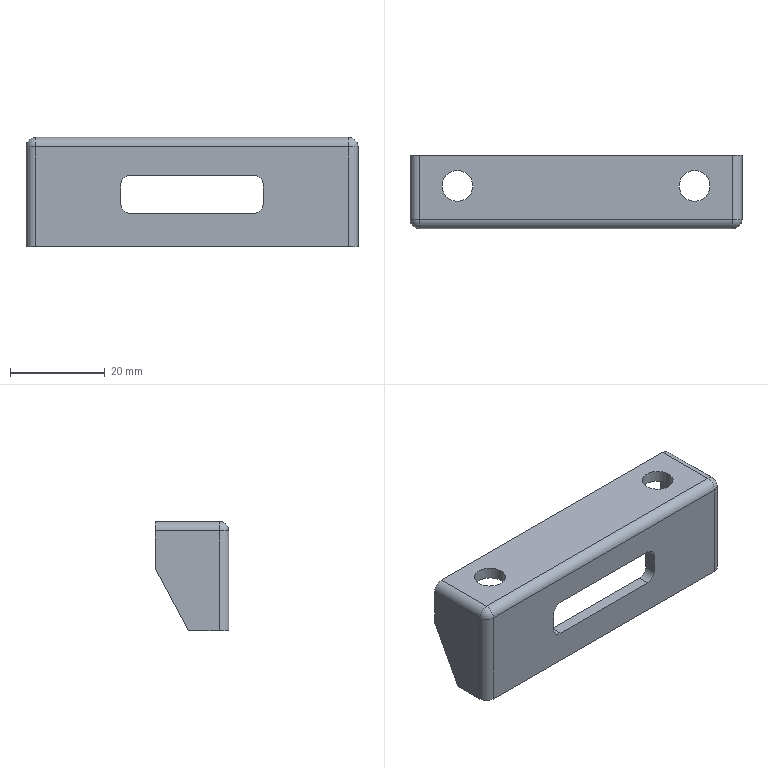Part | NX | features BREP 1 | 1 solid | 31 faces | box 70 x 15.5 x 23 mm | volume 6522 mm3 | plane 16 | cylinder 13 | sphere 2 | commonest cylinder face diameters 4 x9 6.5 x4
STEP:
#1=CARTESIAN_POINT('',(-26.75,9.,11.5));
#2=VERTEX_POINT('',#1);
#3=CARTESIAN_POINT('',(-33.25,9.,11.5));
#4=VERTEX_POINT('',#3);
#5=CARTESIAN_POINT('',(-30.,9.,11.5));
#6=DIRECTION('',(0.,0.,-1.));
#7=DIRECTION('',(-1.,0.,0.));
#8=AXIS2_PLACEMENT_3D('',#5,#6,#7);
#9=CIRCLE('',#8,3.25);
#10=EDGE_CURVE('',#2,#4,#9,.T.);
#11=ORIENTED_EDGE('',*,*,#10,.F.);
#12=CARTESIAN_POINT('',(-26.75,9.,9.));
#13=VERTEX_POINT('',#12);
#14=CARTESIAN_POINT('',(-26.75,9.,9.));
#15=DIRECTION('',(0.,0.,-1.));
#16=VECTOR('',#15,1000.);
#17=LINE('',#14,#16);
#18=EDGE_CURVE('',#13,#2,#17,.F.);
#19=ORIENTED_EDGE('',*,*,#18,.F.);
#20=CARTESIAN_POINT('',(-33.25,9.,9.));
#21=VERTEX_POINT('',#20);
#22=CARTESIAN_POINT('',(-30.,9.,9.));
#23=DIRECTION('',(0.,0.,1.));
#24=DIRECTION('',(-1.,0.,0.));
#25=AXIS2_PLACEMENT_3D('',#22,#23,#24);
#26=CIRCLE('',#25,3.25);
#27=EDGE_CURVE('',#21,#13,#26,.T.);
#28=ORIENTED_EDGE('',*,*,#27,.F.);
#29=CARTESIAN_POINT('',(-33.25,9.,9.));
#30=DIRECTION('',(0.,0.,-1.));
#31=VECTOR('',#30,1000.);
#32=LINE('',#29,#31);
#33=EDGE_CURVE('',#21,#4,#32,.F.);
#34=ORIENTED_EDGE('',*,*,#33,.T.);
#35=EDGE_LOOP('',(#11,#19,#28,#34));
#36=FACE_BOUND('',#35,.T.);
#37=CARTESIAN_POINT('',(-30.,9.,9.));
#38=DIRECTION('',(0.,0.,-1.));
#39=DIRECTION('',(1.,0.,0.));
#40=AXIS2_PLACEMENT_3D('',#37,#38,#39);
#41=CYLINDRICAL_SURFACE('',#40,3.25);
#42=ADVANCED_FACE('',(#36),#41,.F.);
#43=CARTESIAN_POINT('',(23.25,9.,11.5));
#44=VERTEX_POINT('',#43);
#45=CARTESIAN_POINT('',(16.75,9.,11.5));
#46=VERTEX_POINT('',#45);
#47=CARTESIAN_POINT('',(20.,9.,11.5));
#48=DIRECTION('',(0.,0.,-1.));
#49=DIRECTION('',(-1.,0.,0.));
#50=AXIS2_PLACEMENT_3D('',#47,#48,#49);
#51=CIRCLE('',#50,3.25);
#52=EDGE_CURVE('',#44,#46,#51,.T.);
#53=ORIENTED_EDGE('',*,*,#52,.F.);
#54=CARTESIAN_POINT('',(23.25,9.,9.));
#55=VERTEX_POINT('',#54);
#56=CARTESIAN_POINT('',(23.25,9.,9.));
#57=DIRECTION('',(0.,0.,-1.));
#58=VECTOR('',#57,1000.);
#59=LINE('',#56,#58);
#60=EDGE_CURVE('',#55,#44,#59,.F.);
#61=ORIENTED_EDGE('',*,*,#60,.F.);
#62=CARTESIAN_POINT('',(16.75,9.,9.));
#63=VERTEX_POINT('',#62);
#64=CARTESIAN_POINT('',(20.,9.,9.));
#65=DIRECTION('',(0.,0.,1.));
#66=DIRECTION('',(-1.,0.,0.));
#67=AXIS2_PLACEMENT_3D('',#64,#65,#66);
#68=CIRCLE('',#67,3.25);
#69=EDGE_CURVE('',#63,#55,#68,.T.);
#70=ORIENTED_EDGE('',*,*,#69,.F.);
#71=CARTESIAN_POINT('',(16.75,9.,9.));
#72=DIRECTION('',(0.,0.,-1.));
#73=VECTOR('',#72,1000.);
#74=LINE('',#71,#73);
#75=EDGE_CURVE('',#63,#46,#74,.F.);
#76=ORIENTED_EDGE('',*,*,#75,.T.);
#77=EDGE_LOOP('',(#53,#61,#70,#76));
#78=FACE_BOUND('',#77,.T.);
#79=CARTESIAN_POINT('',(20.,9.,9.));
#80=DIRECTION('',(0.,0.,-1.));
#81=DIRECTION('',(1.,0.,0.));
#82=AXIS2_PLACEMENT_3D('',#79,#80,#81);
#83=CYLINDRICAL_SURFACE('',#82,3.25);
#84=ADVANCED_FACE('',(#78),#83,.F.);
#85=CARTESIAN_POINT('',(-38.,0.,9.5));
#86=VERTEX_POINT('',#85);
#87=CARTESIAN_POINT('',(28.,0.,9.5));
#88=VERTEX_POINT('',#87);
#89=CARTESIAN_POINT('',(0.,0.,9.5));
#90=DIRECTION('',(1.,0.,0.));
#91=VECTOR('',#90,1000.);
#92=LINE('',#89,#91);
#93=EDGE_CURVE('',#86,#88,#92,.T.);
#94=ORIENTED_EDGE('',*,*,#93,.F.);
#95=CARTESIAN_POINT('',(-38.,0.,-11.5));
#96=VERTEX_POINT('',#95);
#97=CARTESIAN_POINT('',(-38.,0.,0.));
#98=DIRECTION('',(0.,0.,1.));
#99=VECTOR('',#98,1000.);
#100=LINE('',#97,#99);
#101=EDGE_CURVE('',#96,#86,#100,.T.);
#102=ORIENTED_EDGE('',*,*,#101,.F.);
#103=CARTESIAN_POINT('',(28.,0.,-11.5));
#104=VERTEX_POINT('',#103);
#105=CARTESIAN_POINT('',(0.,0.,-11.5));
#106=DIRECTION('',(-1.,0.,0.));
#107=VECTOR('',#106,1000.);
#108=LINE('',#105,#107);
#109=EDGE_CURVE('',#104,#96,#108,.T.);
#110=ORIENTED_EDGE('',*,*,#109,.F.);
#111=CARTESIAN_POINT('',(28.,0.,0.));
#112=DIRECTION('',(0.,0.,-1.));
#113=VECTOR('',#112,1000.);
#114=LINE('',#111,#113);
#115=EDGE_CURVE('',#88,#104,#114,.T.);
#116=ORIENTED_EDGE('',*,*,#115,.F.);
#117=EDGE_LOOP('',(#94,#102,#110,#116));
#118=FACE_BOUND('',#117,.T.);
#119=CARTESIAN_POINT('',(10.,0.,1.5));
#120=VERTEX_POINT('',#119);
#121=CARTESIAN_POINT('',(8.,0.,3.5));
#122=VERTEX_POINT('',#121);
#123=CARTESIAN_POINT('',(8.,0.,1.5));
#124=DIRECTION('',(0.,-1.,0.));
#125=DIRECTION('',(0.,0.,-1.));
#126=AXIS2_PLACEMENT_3D('',#123,#124,#125);
#127=CIRCLE('',#126,2.);
#128=EDGE_CURVE('',#120,#122,#127,.T.);
#129=ORIENTED_EDGE('',*,*,#128,.F.);
#130=CARTESIAN_POINT('',(10.,0.,-2.5));
#131=VERTEX_POINT('',#130);
#132=CARTESIAN_POINT('',(10.,0.,0.));
#133=DIRECTION('',(0.,0.,1.));
#134=VECTOR('',#133,1000.);
#135=LINE('',#132,#134);
#136=EDGE_CURVE('',#131,#120,#135,.T.);
#137=ORIENTED_EDGE('',*,*,#136,.F.);
#138=CARTESIAN_POINT('',(8.,0.,-4.5));
#139=VERTEX_POINT('',#138);
#140=CARTESIAN_POINT('',(8.,0.,-2.5));
#141=DIRECTION('',(0.,-1.,0.));
#142=DIRECTION('',(0.,0.,-1.));
#143=AXIS2_PLACEMENT_3D('',#140,#141,#142);
#144=CIRCLE('',#143,2.);
#145=EDGE_CURVE('',#139,#131,#144,.T.);
#146=ORIENTED_EDGE('',*,*,#145,.F.);
#147=CARTESIAN_POINT('',(-18.,0.,-4.5));
#148=VERTEX_POINT('',#147);
#149=CARTESIAN_POINT('',(0.,0.,-4.5));
#150=DIRECTION('',(1.,0.,0.));
#151=VECTOR('',#150,1000.);
#152=LINE('',#149,#151);
#153=EDGE_CURVE('',#148,#139,#152,.T.);
#154=ORIENTED_EDGE('',*,*,#153,.F.);
#155=CARTESIAN_POINT('',(-20.,0.,-2.5));
#156=VERTEX_POINT('',#155);
#157=CARTESIAN_POINT('',(-18.,0.,-2.5));
#158=DIRECTION('',(0.,-1.,0.));
#159=DIRECTION('',(0.,0.,-1.));
#160=AXIS2_PLACEMENT_3D('',#157,#158,#159);
#161=CIRCLE('',#160,2.);
#162=EDGE_CURVE('',#156,#148,#161,.T.);
#163=ORIENTED_EDGE('',*,*,#162,.F.);
#164=CARTESIAN_POINT('',(-20.,0.,1.5));
#165=VERTEX_POINT('',#164);
#166=CARTESIAN_POINT('',(-20.,0.,0.));
#167=DIRECTION('',(0.,0.,-1.));
#168=VECTOR('',#167,1000.);
#169=LINE('',#166,#168);
#170=EDGE_CURVE('',#165,#156,#169,.T.);
#171=ORIENTED_EDGE('',*,*,#170,.F.);
#172=CARTESIAN_POINT('',(-18.,0.,3.5));
#173=VERTEX_POINT('',#172);
#174=CARTESIAN_POINT('',(-18.,0.,1.5));
#175=DIRECTION('',(0.,-1.,0.));
#176=DIRECTION('',(0.,0.,-1.));
#177=AXIS2_PLACEMENT_3D('',#174,#175,#176);
#178=CIRCLE('',#177,2.);
#179=EDGE_CURVE('',#173,#165,#178,.T.);
#180=ORIENTED_EDGE('',*,*,#179,.F.);
#181=CARTESIAN_POINT('',(0.,0.,3.5));
#182=DIRECTION('',(-1.,0.,0.));
#183=VECTOR('',#182,1000.);
#184=LINE('',#181,#183);
#185=EDGE_CURVE('',#122,#173,#184,.T.);
#186=ORIENTED_EDGE('',*,*,#185,.F.);
#187=EDGE_LOOP('',(#129,#137,#146,#154,#163,#171,#180,#186));
#188=FACE_BOUND('',#187,.T.);
#189=CARTESIAN_POINT('',(0.,0.,0.));
#190=DIRECTION('',(0.,1.,0.));
#191=DIRECTION('',(0.,0.,-1.));
#192=AXIS2_PLACEMENT_3D('',#189,#190,#191);
#193=PLANE('',#192);
#194=ADVANCED_FACE('',(#118,#188),#193,.F.);
#195=CARTESIAN_POINT('',(30.,2.,-11.5));
#196=VERTEX_POINT('',#195);
#197=CARTESIAN_POINT('',(28.,2.,-11.5));
#198=DIRECTION('',(0.,0.,1.));
#199=DIRECTION('',(1.,0.,0.));
#200=AXIS2_PLACEMENT_3D('',#197,#198,#199);
#201=CIRCLE('',#200,2.);
#202=EDGE_CURVE('',#104,#196,#201,.T.);
#203=ORIENTED_EDGE('',*,*,#202,.T.);
#204=CARTESIAN_POINT('',(30.,2.,9.5));
#205=VERTEX_POINT('',#204);
#206=CARTESIAN_POINT('',(30.,2.,-41.483));
#207=DIRECTION('',(0.,0.,1.));
#208=VECTOR('',#207,1000.);
#209=LINE('',#206,#208);
#210=EDGE_CURVE('',#196,#205,#209,.T.);
#211=ORIENTED_EDGE('',*,*,#210,.T.);
#212=CARTESIAN_POINT('',(28.,2.,9.5));
#213=DIRECTION('',(0.,0.,-1.));
#214=DIRECTION('',(1.,0.,0.));
#215=AXIS2_PLACEMENT_3D('',#212,#213,#214);
#216=CIRCLE('',#215,2.);
#217=EDGE_CURVE('',#205,#88,#216,.T.);
#218=ORIENTED_EDGE('',*,*,#217,.T.);
#219=ORIENTED_EDGE('',*,*,#115,.T.);
#220=EDGE_LOOP('',(#203,#211,#218,#219));
#221=FACE_BOUND('',#220,.T.);
#222=CARTESIAN_POINT('',(28.,2.,-41.483));
#223=DIRECTION('',(0.,0.,1.));
#224=DIRECTION('',(-1.,0.,0.));
#225=AXIS2_PLACEMENT_3D('',#222,#223,#224);
#226=CYLINDRICAL_SURFACE('',#225,2.);
#227=ADVANCED_FACE('',(#221),#226,.T.);
#228=ORIENTED_EDGE('',*,*,#93,.T.);
#229=CARTESIAN_POINT('',(28.,2.,11.5));
#230=VERTEX_POINT('',#229);
#231=CARTESIAN_POINT('',(28.,2.,9.5));
#232=DIRECTION('',(-1.,0.,0.));
#233=DIRECTION('',(0.,0.,1.));
#234=AXIS2_PLACEMENT_3D('',#231,#232,#233);
#235=CIRCLE('',#234,2.);
#236=EDGE_CURVE('',#88,#230,#235,.T.);
#237=ORIENTED_EDGE('',*,*,#236,.T.);
#238=CARTESIAN_POINT('',(-38.,2.,11.5));
#239=VERTEX_POINT('',#238);
#240=CARTESIAN_POINT('',(108.216,2.,11.5));
#241=DIRECTION('',(-1.,0.,0.));
#242=VECTOR('',#241,1000.);
#243=LINE('',#240,#242);
#244=EDGE_CURVE('',#230,#239,#243,.T.);
#245=ORIENTED_EDGE('',*,*,#244,.T.);
#246=CARTESIAN_POINT('',(-38.,2.,9.5));
#247=DIRECTION('',(1.,0.,0.));
#248=DIRECTION('',(0.,0.,1.));
#249=AXIS2_PLACEMENT_3D('',#246,#247,#248);
#250=CIRCLE('',#249,2.);
#251=EDGE_CURVE('',#239,#86,#250,.T.);
#252=ORIENTED_EDGE('',*,*,#251,.T.);
#253=EDGE_LOOP('',(#228,#237,#245,#252));
#254=FACE_BOUND('',#253,.T.);
#255=CARTESIAN_POINT('',(108.216,2.,9.5));
#256=DIRECTION('',(-1.,0.,0.));
#257=DIRECTION('',(0.,0.,-1.));
#258=AXIS2_PLACEMENT_3D('',#255,#256,#257);
#259=CYLINDRICAL_SURFACE('',#258,2.);
#260=ADVANCED_FACE('',(#254),#259,.T.);
#261=ORIENTED_EDGE('',*,*,#101,.T.);
#262=CARTESIAN_POINT('',(-40.,2.,9.5));
#263=VERTEX_POINT('',#262);
#264=CARTESIAN_POINT('',(-38.,2.,9.5));
#265=DIRECTION('',(0.,0.,-1.));
#266=DIRECTION('',(1.,0.,0.));
#267=AXIS2_PLACEMENT_3D('',#264,#265,#266);
#268=CIRCLE('',#267,2.);
#269=EDGE_CURVE('',#86,#263,#268,.T.);
#270=ORIENTED_EDGE('',*,*,#269,.T.);
#271=CARTESIAN_POINT('',(-40.,2.,-11.5));
#272=VERTEX_POINT('',#271);
#273=CARTESIAN_POINT('',(-40.,2.,-41.483));
#274=DIRECTION('',(0.,0.,-1.));
#275=VECTOR('',#274,1000.);
#276=LINE('',#273,#275);
#277=EDGE_CURVE('',#263,#272,#276,.T.);
#278=ORIENTED_EDGE('',*,*,#277,.T.);
#279=CARTESIAN_POINT('',(-38.,2.,-11.5));
#280=DIRECTION('',(0.,0.,1.));
#281=DIRECTION('',(1.,0.,0.));
#282=AXIS2_PLACEMENT_3D('',#279,#280,#281);
#283=CIRCLE('',#282,2.);
#284=EDGE_CURVE('',#272,#96,#283,.T.);
#285=ORIENTED_EDGE('',*,*,#284,.T.);
#286=EDGE_LOOP('',(#261,#270,#278,#285));
#287=FACE_BOUND('',#286,.T.);
#288=CARTESIAN_POINT('',(-38.,2.,-41.483));
#289=DIRECTION('',(0.,0.,1.));
#290=DIRECTION('',(-1.,0.,0.));
#291=AXIS2_PLACEMENT_3D('',#288,#289,#290);
#292=CYLINDRICAL_SURFACE('',#291,2.);
#293=ADVANCED_FACE('',(#287),#292,.T.);
#294=CARTESIAN_POINT('',(30.,8.5,-11.5));
#295=VERTEX_POINT('',#294);
#296=CARTESIAN_POINT('',(30.,0.,-11.5));
#297=DIRECTION('',(0.,-1.,0.));
#298=VECTOR('',#297,1000.);
#299=LINE('',#296,#298);
#300=EDGE_CURVE('',#295,#196,#299,.T.);
#301=ORIENTED_EDGE('',*,*,#300,.T.);
#302=ORIENTED_EDGE('',*,*,#202,.F.);
#303=ORIENTED_EDGE('',*,*,#109,.T.);
#304=ORIENTED_EDGE('',*,*,#284,.F.);
#305=CARTESIAN_POINT('',(-40.,8.5,-11.5));
#306=VERTEX_POINT('',#305);
#307=CARTESIAN_POINT('',(-40.,0.,-11.5));
#308=DIRECTION('',(0.,1.,0.));
#309=VECTOR('',#308,1000.);
#310=LINE('',#307,#309);
#311=EDGE_CURVE('',#272,#306,#310,.T.);
#312=ORIENTED_EDGE('',*,*,#311,.T.);
#313=CARTESIAN_POINT('',(-37.5,8.5,-11.5));
#314=VERTEX_POINT('',#313);
#315=CARTESIAN_POINT('',(30.,8.5,-11.5));
#316=DIRECTION('',(1.,0.,0.));
#317=VECTOR('',#316,1000.);
#318=LINE('',#315,#317);
#319=EDGE_CURVE('',#306,#314,#318,.T.);
#320=ORIENTED_EDGE('',*,*,#319,.T.);
#321=CARTESIAN_POINT('',(-37.5,2.5,-11.5));
#322=VERTEX_POINT('',#321);
#323=CARTESIAN_POINT('',(-37.5,0.,-11.5));
#324=DIRECTION('',(0.,-1.,0.));
#325=VECTOR('',#324,1000.);
#326=LINE('',#323,#325);
#327=EDGE_CURVE('',#314,#322,#326,.T.);
#328=ORIENTED_EDGE('',*,*,#327,.T.);
#329=CARTESIAN_POINT('',(27.5,2.5,-11.5));
#330=VERTEX_POINT('',#329);
#331=CARTESIAN_POINT('',(30.,2.5,-11.5));
#332=DIRECTION('',(1.,0.,0.));
#333=VECTOR('',#332,1000.);
#334=LINE('',#331,#333);
#335=EDGE_CURVE('',#322,#330,#334,.T.);
#336=ORIENTED_EDGE('',*,*,#335,.T.);
#337=CARTESIAN_POINT('',(27.5,8.5,-11.5));
#338=VERTEX_POINT('',#337);
#339=CARTESIAN_POINT('',(27.5,0.,-11.5));
#340=DIRECTION('',(0.,1.,0.));
#341=VECTOR('',#340,1000.);
#342=LINE('',#339,#341);
#343=EDGE_CURVE('',#330,#338,#342,.T.);
#344=ORIENTED_EDGE('',*,*,#343,.T.);
#345=CARTESIAN_POINT('',(30.,8.5,-11.5));
#346=DIRECTION('',(1.,0.,0.));
#347=VECTOR('',#346,1000.);
#348=LINE('',#345,#347);
#349=EDGE_CURVE('',#338,#295,#348,.T.);
#350=ORIENTED_EDGE('',*,*,#349,.T.);
#351=EDGE_LOOP('',(#301,#302,#303,#304,#312,#320,#328,#336,#344,#350));
#352=FACE_BOUND('',#351,.T.);
#353=CARTESIAN_POINT('',(30.,0.,-11.5));
#354=DIRECTION('',(0.,0.,-1.));
#355=DIRECTION('',(1.,0.,0.));
#356=AXIS2_PLACEMENT_3D('',#353,#354,#355);
#357=PLANE('',#356);
#358=ADVANCED_FACE('',(#352),#357,.T.);
#359=ORIENTED_EDGE('',*,*,#185,.T.);
#360=CARTESIAN_POINT('',(-18.,2.5,3.5));
#361=VERTEX_POINT('',#360);
#362=CARTESIAN_POINT('',(-18.,2.5,3.5));
#363=DIRECTION('',(0.,-1.,0.));
#364=VECTOR('',#363,1000.);
#365=LINE('',#362,#364);
#366=EDGE_CURVE('',#361,#173,#365,.T.);
#367=ORIENTED_EDGE('',*,*,#366,.F.);
#368=CARTESIAN_POINT('',(8.,2.5,3.5));
#369=VERTEX_POINT('',#368);
#370=CARTESIAN_POINT('',(-10.,2.5,3.5));
#371=DIRECTION('',(-1.,0.,0.));
#372=VECTOR('',#371,1000.);
#373=LINE('',#370,#372);
#374=EDGE_CURVE('',#369,#361,#373,.T.);
#375=ORIENTED_EDGE('',*,*,#374,.F.);
#376=CARTESIAN_POINT('',(8.,2.5,3.5));
#377=DIRECTION('',(0.,1.,0.));
#378=VECTOR('',#377,1000.);
#379=LINE('',#376,#378);
#380=EDGE_CURVE('',#122,#369,#379,.T.);
#381=ORIENTED_EDGE('',*,*,#380,.F.);
#382=EDGE_LOOP('',(#359,#367,#375,#381));
#383=FACE_BOUND('',#382,.T.);
#384=CARTESIAN_POINT('',(-10.,2.5,3.5));
#385=DIRECTION('',(0.,0.,1.));
#386=DIRECTION('',(-1.,0.,0.));
#387=AXIS2_PLACEMENT_3D('',#384,#385,#386);
#388=PLANE('',#387);
#389=ADVANCED_FACE('',(#383),#388,.F.);
#390=CARTESIAN_POINT('',(10.,2.5,1.5));
#391=VERTEX_POINT('',#390);
#392=CARTESIAN_POINT('',(8.,2.5,1.5));
#393=DIRECTION('',(0.,-1.,0.));
#394=DIRECTION('',(0.,0.,-1.));
#395=AXIS2_PLACEMENT_3D('',#392,#393,#394);
#396=CIRCLE('',#395,2.);
#397=EDGE_CURVE('',#391,#369,#396,.T.);
#398=ORIENTED_EDGE('',*,*,#397,.F.);
#399=CARTESIAN_POINT('',(10.,38.009,1.5));
#400=DIRECTION('',(0.,1.,0.));
#401=VECTOR('',#400,1000.);
#402=LINE('',#399,#401);
#403=EDGE_CURVE('',#120,#391,#402,.T.);
#404=ORIENTED_EDGE('',*,*,#403,.F.);
#405=ORIENTED_EDGE('',*,*,#128,.T.);
#406=ORIENTED_EDGE('',*,*,#380,.T.);
#407=EDGE_LOOP('',(#398,#404,#405,#406));
#408=FACE_BOUND('',#407,.T.);
#409=CARTESIAN_POINT('',(8.,38.009,1.5));
#410=DIRECTION('',(0.,-1.,0.));
#411=DIRECTION('',(0.,0.,1.));
#412=AXIS2_PLACEMENT_3D('',#409,#410,#411);
#413=CYLINDRICAL_SURFACE('',#412,2.);
#414=ADVANCED_FACE('',(#408),#413,.F.);
#415=CARTESIAN_POINT('',(10.,2.5,-2.5));
#416=VERTEX_POINT('',#415);
#417=CARTESIAN_POINT('',(10.,2.5,3.5));
#418=DIRECTION('',(0.,0.,1.));
#419=VECTOR('',#418,1000.);
#420=LINE('',#417,#419);
#421=EDGE_CURVE('',#416,#391,#420,.T.);
#422=ORIENTED_EDGE('',*,*,#421,.F.);
#423=CARTESIAN_POINT('',(10.,2.5,-2.5));
#424=DIRECTION('',(0.,1.,0.));
#425=VECTOR('',#424,1000.);
#426=LINE('',#423,#425);
#427=EDGE_CURVE('',#131,#416,#426,.T.);
#428=ORIENTED_EDGE('',*,*,#427,.F.);
#429=ORIENTED_EDGE('',*,*,#136,.T.);
#430=ORIENTED_EDGE('',*,*,#403,.T.);
#431=EDGE_LOOP('',(#422,#428,#429,#430));
#432=FACE_BOUND('',#431,.T.);
#433=CARTESIAN_POINT('',(10.,2.5,3.5));
#434=DIRECTION('',(1.,0.,0.));
#435=DIRECTION('',(0.,0.,1.));
#436=AXIS2_PLACEMENT_3D('',#433,#434,#435);
#437=PLANE('',#436);
#438=ADVANCED_FACE('',(#432),#437,.F.);
#439=CARTESIAN_POINT('',(8.,2.5,-4.5));
#440=VERTEX_POINT('',#439);
#441=CARTESIAN_POINT('',(8.,2.5,-2.5));
#442=DIRECTION('',(0.,-1.,0.));
#443=DIRECTION('',(0.,0.,-1.));
#444=AXIS2_PLACEMENT_3D('',#441,#442,#443);
#445=CIRCLE('',#444,2.);
#446=EDGE_CURVE('',#440,#416,#445,.T.);
#447=ORIENTED_EDGE('',*,*,#446,.F.);
#448=CARTESIAN_POINT('',(8.,38.009,-4.5));
#449=DIRECTION('',(0.,1.,0.));
#450=VECTOR('',#449,1000.);
#451=LINE('',#448,#450);
#452=EDGE_CURVE('',#139,#440,#451,.T.);
#453=ORIENTED_EDGE('',*,*,#452,.F.);
#454=ORIENTED_EDGE('',*,*,#145,.T.);
#455=ORIENTED_EDGE('',*,*,#427,.T.);
#456=EDGE_LOOP('',(#447,#453,#454,#455));
#457=FACE_BOUND('',#456,.T.);
#458=CARTESIAN_POINT('',(8.,38.009,-2.5));
#459=DIRECTION('',(0.,-1.,0.));
#460=DIRECTION('',(0.,0.,1.));
#461=AXIS2_PLACEMENT_3D('',#458,#459,#460);
#462=CYLINDRICAL_SURFACE('',#461,2.);
#463=ADVANCED_FACE('',(#457),#462,.F.);
#464=CARTESIAN_POINT('',(-18.,2.5,-4.5));
#465=VERTEX_POINT('',#464);
#466=CARTESIAN_POINT('',(10.,2.5,-4.5));
#467=DIRECTION('',(1.,0.,0.));
#468=VECTOR('',#467,1000.);
#469=LINE('',#466,#468);
#470=EDGE_CURVE('',#465,#440,#469,.T.);
#471=ORIENTED_EDGE('',*,*,#470,.F.);
#472=CARTESIAN_POINT('',(-18.,2.5,-4.5));
#473=DIRECTION('',(0.,1.,0.));
#474=VECTOR('',#473,1000.);
#475=LINE('',#472,#474);
#476=EDGE_CURVE('',#148,#465,#475,.T.);
#477=ORIENTED_EDGE('',*,*,#476,.F.);
#478=ORIENTED_EDGE('',*,*,#153,.T.);
#479=ORIENTED_EDGE('',*,*,#452,.T.);
#480=EDGE_LOOP('',(#471,#477,#478,#479));
#481=FACE_BOUND('',#480,.T.);
#482=CARTESIAN_POINT('',(10.,2.5,-4.5));
#483=DIRECTION('',(0.,0.,-1.));
#484=DIRECTION('',(1.,0.,0.));
#485=AXIS2_PLACEMENT_3D('',#482,#483,#484);
#486=PLANE('',#485);
#487=ADVANCED_FACE('',(#481),#486,.F.);
#488=CARTESIAN_POINT('',(-20.,2.5,-2.5));
#489=VERTEX_POINT('',#488);
#490=CARTESIAN_POINT('',(-18.,2.5,-2.5));
#491=DIRECTION('',(0.,-1.,0.));
#492=DIRECTION('',(0.,0.,-1.));
#493=AXIS2_PLACEMENT_3D('',#490,#491,#492);
#494=CIRCLE('',#493,2.);
#495=EDGE_CURVE('',#489,#465,#494,.T.);
#496=ORIENTED_EDGE('',*,*,#495,.F.);
#497=CARTESIAN_POINT('',(-20.,38.009,-2.5));
#498=DIRECTION('',(0.,1.,0.));
#499=VECTOR('',#498,1000.);
#500=LINE('',#497,#499);
#501=EDGE_CURVE('',#156,#489,#500,.T.);
#502=ORIENTED_EDGE('',*,*,#501,.F.);
#503=ORIENTED_EDGE('',*,*,#162,.T.);
#504=ORIENTED_EDGE('',*,*,#476,.T.);
#505=EDGE_LOOP('',(#496,#502,#503,#504));
#506=FACE_BOUND('',#505,.T.);
#507=CARTESIAN_POINT('',(-18.,38.009,-2.5));
#508=DIRECTION('',(0.,-1.,0.));
#509=DIRECTION('',(0.,0.,1.));
#510=AXIS2_PLACEMENT_3D('',#507,#508,#509);
#511=CYLINDRICAL_SURFACE('',#510,2.);
#512=ADVANCED_FACE('',(#506),#511,.F.);
#513=CARTESIAN_POINT('',(-20.,2.5,1.5));
#514=VERTEX_POINT('',#513);
#515=CARTESIAN_POINT('',(-20.,2.5,-4.5));
#516=DIRECTION('',(0.,0.,-1.));
#517=VECTOR('',#516,1000.);
#518=LINE('',#515,#517);
#519=EDGE_CURVE('',#514,#489,#518,.T.);
#520=ORIENTED_EDGE('',*,*,#519,.F.);
#521=CARTESIAN_POINT('',(-20.,2.5,1.5));
#522=DIRECTION('',(0.,1.,0.));
#523=VECTOR('',#522,1000.);
#524=LINE('',#521,#523);
#525=EDGE_CURVE('',#165,#514,#524,.T.);
#526=ORIENTED_EDGE('',*,*,#525,.F.);
#527=ORIENTED_EDGE('',*,*,#170,.T.);
#528=ORIENTED_EDGE('',*,*,#501,.T.);
#529=EDGE_LOOP('',(#520,#526,#527,#528));
#530=FACE_BOUND('',#529,.T.);
#531=CARTESIAN_POINT('',(-20.,2.5,-4.5));
#532=DIRECTION('',(-1.,0.,0.));
#533=DIRECTION('',(0.,0.,-1.));
#534=AXIS2_PLACEMENT_3D('',#531,#532,#533);
#535=PLANE('',#534);
#536=ADVANCED_FACE('',(#530),#535,.F.);
#537=CARTESIAN_POINT('',(-18.,2.5,1.5));
#538=DIRECTION('',(0.,-1.,0.));
#539=DIRECTION('',(0.,0.,-1.));
#540=AXIS2_PLACEMENT_3D('',#537,#538,#539);
#541=CIRCLE('',#540,2.);
#542=EDGE_CURVE('',#361,#514,#541,.T.);
#543=ORIENTED_EDGE('',*,*,#542,.F.);
#544=ORIENTED_EDGE('',*,*,#366,.T.);
#545=ORIENTED_EDGE('',*,*,#179,.T.);
#546=ORIENTED_EDGE('',*,*,#525,.T.);
#547=EDGE_LOOP('',(#543,#544,#545,#546));
#548=FACE_BOUND('',#547,.T.);
#549=CARTESIAN_POINT('',(-18.,38.009,1.5));
#550=DIRECTION('',(0.,-1.,0.));
#551=DIRECTION('',(0.,0.,1.));
#552=AXIS2_PLACEMENT_3D('',#549,#550,#551);
#553=CYLINDRICAL_SURFACE('',#552,2.);
#554=ADVANCED_FACE('',(#548),#553,.F.);
#555=CARTESIAN_POINT('',(30.,15.5,9.5));
#556=VERTEX_POINT('',#555);
#557=CARTESIAN_POINT('',(30.,0.,9.5));
#558=DIRECTION('',(0.,-1.,0.));
#559=VECTOR('',#558,1000.);
#560=LINE('',#557,#559);
#561=EDGE_CURVE('',#556,#205,#560,.T.);
#562=ORIENTED_EDGE('',*,*,#561,.T.);
#563=ORIENTED_EDGE('',*,*,#210,.F.);
#564=ORIENTED_EDGE('',*,*,#300,.F.);
#565=CARTESIAN_POINT('',(30.,15.5,1.625));
#566=VERTEX_POINT('',#565);
#567=CARTESIAN_POINT('',(30.,8.5,-11.5));
#568=DIRECTION('',(0.,0.4706,0.8824));
#569=VECTOR('',#568,1000.);
#570=LINE('',#567,#569);
#571=EDGE_CURVE('',#295,#566,#570,.T.);
#572=ORIENTED_EDGE('',*,*,#571,.T.);
#573=CARTESIAN_POINT('',(30.,15.5,11.5));
#574=DIRECTION('',(0.,0.,1.));
#575=VECTOR('',#574,1000.);
#576=LINE('',#573,#575);
#577=EDGE_CURVE('',#566,#556,#576,.T.);
#578=ORIENTED_EDGE('',*,*,#577,.T.);
#579=EDGE_LOOP('',(#562,#563,#564,#572,#578));
#580=FACE_BOUND('',#579,.T.);
#581=CARTESIAN_POINT('',(30.,0.,11.5));
#582=DIRECTION('',(1.,0.,0.));
#583=DIRECTION('',(0.,0.,1.));
#584=AXIS2_PLACEMENT_3D('',#581,#582,#583);
#585=PLANE('',#584);
#586=ADVANCED_FACE('',(#580),#585,.T.);
#587=ORIENTED_EDGE('',*,*,#217,.F.);
#588=CARTESIAN_POINT('',(28.,2.,9.5));
#589=DIRECTION('',(0.,-1.,0.));
#590=DIRECTION('',(1.,0.,0.));
#591=AXIS2_PLACEMENT_3D('',#588,#589,#590);
#592=CIRCLE('',#591,2.);
#593=EDGE_CURVE('',#205,#230,#592,.T.);
#594=ORIENTED_EDGE('',*,*,#593,.T.);
#595=ORIENTED_EDGE('',*,*,#236,.F.);
#596=EDGE_LOOP('',(#587,#594,#595));
#597=FACE_BOUND('',#596,.T.);
#598=CARTESIAN_POINT('',(28.,2.,9.5));
#599=DIRECTION('',(0.,0.,1.));
#600=DIRECTION('',(-1.,0.,0.));
#601=AXIS2_PLACEMENT_3D('',#598,#599,#600);
#602=SPHERICAL_SURFACE('',#601,2.);
#603=ADVANCED_FACE('',(#597),#602,.T.);
#604=ORIENTED_EDGE('',*,*,#251,.F.);
#605=CARTESIAN_POINT('',(-38.,2.,9.5));
#606=DIRECTION('',(-0.000000002,-1.,0.));
#607=DIRECTION('',(0.,0.,1.));
#608=AXIS2_PLACEMENT_3D('',#605,#606,#607);
#609=CIRCLE('',#608,2.);
#610=EDGE_CURVE('',#239,#263,#609,.T.);
#611=ORIENTED_EDGE('',*,*,#610,.T.);
#612=ORIENTED_EDGE('',*,*,#269,.F.);
#613=EDGE_LOOP('',(#604,#611,#612));
#614=FACE_BOUND('',#613,.T.);
#615=CARTESIAN_POINT('',(-38.,2.,9.5));
#616=DIRECTION('',(0.000000002,1.,0.));
#617=DIRECTION('',(-1.,0.000000002,0.));
#618=AXIS2_PLACEMENT_3D('',#615,#616,#617);
#619=SPHERICAL_SURFACE('',#618,2.);
#620=ADVANCED_FACE('',(#614),#619,.T.);
#621=ORIENTED_EDGE('',*,*,#244,.F.);
#622=CARTESIAN_POINT('',(28.,15.5,11.5));
#623=VERTEX_POINT('',#622);
#624=CARTESIAN_POINT('',(28.,0.,11.5));
#625=DIRECTION('',(0.,1.,0.));
#626=VECTOR('',#625,1000.);
#627=LINE('',#624,#626);
#628=EDGE_CURVE('',#230,#623,#627,.T.);
#629=ORIENTED_EDGE('',*,*,#628,.T.);
#630=CARTESIAN_POINT('',(-38.,15.5,11.5));
#631=VERTEX_POINT('',#630);
#632=CARTESIAN_POINT('',(-30.,15.5,11.5));
#633=DIRECTION('',(-1.,0.,0.));
#634=VECTOR('',#633,1000.);
#635=LINE('',#632,#634);
#636=EDGE_CURVE('',#623,#631,#635,.T.);
#637=ORIENTED_EDGE('',*,*,#636,.T.);
#638=CARTESIAN_POINT('',(-38.,0.,11.5));
#639=DIRECTION('',(0.,-1.,0.));
#640=VECTOR('',#639,1000.);
#641=LINE('',#638,#640);
#642=EDGE_CURVE('',#631,#239,#641,.T.);
#643=ORIENTED_EDGE('',*,*,#642,.T.);
#644=EDGE_LOOP('',(#621,#629,#637,#643));
#645=FACE_BOUND('',#644,.T.);
#646=CARTESIAN_POINT('',(-30.,9.,11.5));
#647=DIRECTION('',(0.,0.,-1.));
#648=DIRECTION('',(-1.,0.,0.));
#649=AXIS2_PLACEMENT_3D('',#646,#647,#648);
#650=CIRCLE('',#649,3.25);
#651=EDGE_CURVE('',#4,#2,#650,.T.);
#652=ORIENTED_EDGE('',*,*,#651,.T.);
#653=ORIENTED_EDGE('',*,*,#10,.T.);
#654=EDGE_LOOP('',(#652,#653));
#655=FACE_BOUND('',#654,.T.);
#656=CARTESIAN_POINT('',(20.,9.,11.5));
#657=DIRECTION('',(0.,0.,-1.));
#658=DIRECTION('',(-1.,0.,0.));
#659=AXIS2_PLACEMENT_3D('',#656,#657,#658);
#660=CIRCLE('',#659,3.25);
#661=EDGE_CURVE('',#46,#44,#660,.T.);
#662=ORIENTED_EDGE('',*,*,#661,.T.);
#663=ORIENTED_EDGE('',*,*,#52,.T.);
#664=EDGE_LOOP('',(#662,#663));
#665=FACE_BOUND('',#664,.T.);
#666=CARTESIAN_POINT('',(-30.,0.,11.5));
#667=DIRECTION('',(0.,0.,1.));
#668=DIRECTION('',(-1.,0.,0.));
#669=AXIS2_PLACEMENT_3D('',#666,#667,#668);
#670=PLANE('',#669);
#671=ADVANCED_FACE('',(#645,#655,#665),#670,.T.);
#672=CARTESIAN_POINT('',(-40.,15.5,1.625));
#673=VERTEX_POINT('',#672);
#674=CARTESIAN_POINT('',(-40.,15.5,1.625));
#675=DIRECTION('',(0.,-0.4706,-0.8824));
#676=VECTOR('',#675,1000.);
#677=LINE('',#674,#676);
#678=EDGE_CURVE('',#673,#306,#677,.T.);
#679=ORIENTED_EDGE('',*,*,#678,.T.);
#680=ORIENTED_EDGE('',*,*,#311,.F.);
#681=ORIENTED_EDGE('',*,*,#277,.F.);
#682=CARTESIAN_POINT('',(-40.,15.5,9.5));
#683=VERTEX_POINT('',#682);
#684=CARTESIAN_POINT('',(-40.,0.,9.5));
#685=DIRECTION('',(0.,1.,0.));
#686=VECTOR('',#685,1000.);
#687=LINE('',#684,#686);
#688=EDGE_CURVE('',#263,#683,#687,.T.);
#689=ORIENTED_EDGE('',*,*,#688,.T.);
#690=CARTESIAN_POINT('',(-40.,15.5,-11.5));
#691=DIRECTION('',(0.,0.,-1.));
#692=VECTOR('',#691,1000.);
#693=LINE('',#690,#692);
#694=EDGE_CURVE('',#683,#673,#693,.T.);
#695=ORIENTED_EDGE('',*,*,#694,.T.);
#696=EDGE_LOOP('',(#679,#680,#681,#689,#695));
#697=FACE_BOUND('',#696,.T.);
#698=CARTESIAN_POINT('',(-40.,0.,-11.5));
#699=DIRECTION('',(-1.,0.,0.));
#700=DIRECTION('',(0.,0.,-1.));
#701=AXIS2_PLACEMENT_3D('',#698,#699,#700);
#702=PLANE('',#701);
#703=ADVANCED_FACE('',(#697),#702,.T.);
#704=CARTESIAN_POINT('',(27.5,15.5,1.625));
#705=VERTEX_POINT('',#704);
#706=CARTESIAN_POINT('',(28.75,15.5,1.625));
#707=DIRECTION('',(1.,0.,0.));
#708=VECTOR('',#707,1000.);
#709=LINE('',#706,#708);
#710=EDGE_CURVE('',#705,#566,#709,.T.);
#711=ORIENTED_EDGE('',*,*,#710,.T.);
#712=ORIENTED_EDGE('',*,*,#571,.F.);
#713=ORIENTED_EDGE('',*,*,#349,.F.);
#714=CARTESIAN_POINT('',(27.5,12.5,-4.));
#715=DIRECTION('',(0.,0.4706,0.8824));
#716=VECTOR('',#715,1000.);
#717=LINE('',#714,#716);
#718=EDGE_CURVE('',#338,#705,#717,.T.);
#719=ORIENTED_EDGE('',*,*,#718,.T.);
#720=EDGE_LOOP('',(#711,#712,#713,#719));
#721=FACE_BOUND('',#720,.T.);
#722=CARTESIAN_POINT('',(28.75,12.5,-4.));
#723=DIRECTION('',(0.,0.8824,-0.4706));
#724=DIRECTION('',(0.,-0.4706,-0.8824));
#725=AXIS2_PLACEMENT_3D('',#722,#723,#724);
#726=PLANE('',#725);
#727=ADVANCED_FACE('',(#721),#726,.T.);
#728=CARTESIAN_POINT('',(27.5,15.5,9.));
#729=VERTEX_POINT('',#728);
#730=CARTESIAN_POINT('',(27.5,2.5,9.));
#731=VERTEX_POINT('',#730);
#732=CARTESIAN_POINT('',(27.5,0.,9.));
#733=DIRECTION('',(0.,-1.,0.));
#734=VECTOR('',#733,1000.);
#735=LINE('',#732,#734);
#736=EDGE_CURVE('',#729,#731,#735,.T.);
#737=ORIENTED_EDGE('',*,*,#736,.F.);
#738=CARTESIAN_POINT('',(27.5,15.5,11.5));
#739=DIRECTION('',(0.,0.,1.));
#740=VECTOR('',#739,1000.);
#741=LINE('',#738,#740);
#742=EDGE_CURVE('',#705,#729,#741,.T.);
#743=ORIENTED_EDGE('',*,*,#742,.F.);
#744=ORIENTED_EDGE('',*,*,#718,.F.);
#745=ORIENTED_EDGE('',*,*,#343,.F.);
#746=CARTESIAN_POINT('',(27.5,2.5,11.5));
#747=DIRECTION('',(0.,0.,-1.));
#748=VECTOR('',#747,1000.);
#749=LINE('',#746,#748);
#750=EDGE_CURVE('',#731,#330,#749,.T.);
#751=ORIENTED_EDGE('',*,*,#750,.F.);
#752=EDGE_LOOP('',(#737,#743,#744,#745,#751));
#753=FACE_BOUND('',#752,.T.);
#754=CARTESIAN_POINT('',(27.5,0.,11.5));
#755=DIRECTION('',(1.,0.,0.));
#756=DIRECTION('',(0.,0.,1.));
#757=AXIS2_PLACEMENT_3D('',#754,#755,#756);
#758=PLANE('',#757);
#759=ADVANCED_FACE('',(#753),#758,.F.);
#760=ORIENTED_EDGE('',*,*,#335,.F.);
#761=CARTESIAN_POINT('',(-37.5,2.5,9.));
#762=VERTEX_POINT('',#761);
#763=CARTESIAN_POINT('',(-37.5,2.5,0.));
#764=DIRECTION('',(0.,0.,1.));
#765=VECTOR('',#764,1000.);
#766=LINE('',#763,#765);
#767=EDGE_CURVE('',#322,#762,#766,.T.);
#768=ORIENTED_EDGE('',*,*,#767,.T.);
#769=CARTESIAN_POINT('',(0.,2.5,9.));
#770=DIRECTION('',(1.,0.,0.));
#771=VECTOR('',#770,1000.);
#772=LINE('',#769,#771);
#773=EDGE_CURVE('',#762,#731,#772,.T.);
#774=ORIENTED_EDGE('',*,*,#773,.T.);
#775=ORIENTED_EDGE('',*,*,#750,.T.);
#776=EDGE_LOOP('',(#760,#768,#774,#775));
#777=FACE_BOUND('',#776,.T.);
#778=ORIENTED_EDGE('',*,*,#542,.T.);
#779=ORIENTED_EDGE('',*,*,#519,.T.);
#780=ORIENTED_EDGE('',*,*,#495,.T.);
#781=ORIENTED_EDGE('',*,*,#470,.T.);
#782=ORIENTED_EDGE('',*,*,#446,.T.);
#783=ORIENTED_EDGE('',*,*,#421,.T.);
#784=ORIENTED_EDGE('',*,*,#397,.T.);
#785=ORIENTED_EDGE('',*,*,#374,.T.);
#786=EDGE_LOOP('',(#778,#779,#780,#781,#782,#783,#784,#785));
#787=FACE_BOUND('',#786,.T.);
#788=CARTESIAN_POINT('',(0.,2.5,0.));
#789=DIRECTION('',(0.,1.,0.));
#790=DIRECTION('',(0.,0.,-1.));
#791=AXIS2_PLACEMENT_3D('',#788,#789,#790);
#792=PLANE('',#791);
#793=ADVANCED_FACE('',(#777,#787),#792,.T.);
#794=ORIENTED_EDGE('',*,*,#767,.F.);
#795=ORIENTED_EDGE('',*,*,#327,.F.);
#796=CARTESIAN_POINT('',(-37.5,15.5,1.625));
#797=VERTEX_POINT('',#796);
#798=CARTESIAN_POINT('',(-37.5,15.5,1.625));
#799=DIRECTION('',(0.,-0.4706,-0.8824));
#800=VECTOR('',#799,1000.);
#801=LINE('',#798,#800);
#802=EDGE_CURVE('',#797,#314,#801,.T.);
#803=ORIENTED_EDGE('',*,*,#802,.F.);
#804=CARTESIAN_POINT('',(-37.5,15.5,9.));
#805=VERTEX_POINT('',#804);
#806=CARTESIAN_POINT('',(-37.5,15.5,-11.5));
#807=DIRECTION('',(0.,0.,-1.));
#808=VECTOR('',#807,1000.);
#809=LINE('',#806,#808);
#810=EDGE_CURVE('',#805,#797,#809,.T.);
#811=ORIENTED_EDGE('',*,*,#810,.F.);
#812=CARTESIAN_POINT('',(-37.5,0.,9.));
#813=DIRECTION('',(0.,1.,0.));
#814=VECTOR('',#813,1000.);
#815=LINE('',#812,#814);
#816=EDGE_CURVE('',#762,#805,#815,.T.);
#817=ORIENTED_EDGE('',*,*,#816,.F.);
#818=EDGE_LOOP('',(#794,#795,#803,#811,#817));
#819=FACE_BOUND('',#818,.T.);
#820=CARTESIAN_POINT('',(-37.5,0.,-11.5));
#821=DIRECTION('',(-1.,0.,0.));
#822=DIRECTION('',(0.,0.,-1.));
#823=AXIS2_PLACEMENT_3D('',#820,#821,#822);
#824=PLANE('',#823);
#825=ADVANCED_FACE('',(#819),#824,.F.);
#826=CARTESIAN_POINT('',(28.75,15.5,1.625));
#827=DIRECTION('',(1.,0.,0.));
#828=VECTOR('',#827,1000.);
#829=LINE('',#826,#828);
#830=EDGE_CURVE('',#673,#797,#829,.T.);
#831=ORIENTED_EDGE('',*,*,#830,.T.);
#832=ORIENTED_EDGE('',*,*,#802,.T.);
#833=ORIENTED_EDGE('',*,*,#319,.F.);
#834=ORIENTED_EDGE('',*,*,#678,.F.);
#835=EDGE_LOOP('',(#831,#832,#833,#834));
#836=FACE_BOUND('',#835,.T.);
#837=CARTESIAN_POINT('',(28.75,12.5,-4.));
#838=DIRECTION('',(0.,0.8824,-0.4706));
#839=DIRECTION('',(0.,-0.4706,-0.8824));
#840=AXIS2_PLACEMENT_3D('',#837,#838,#839);
#841=PLANE('',#840);
#842=ADVANCED_FACE('',(#836),#841,.T.);
#843=ORIENTED_EDGE('',*,*,#628,.F.);
#844=ORIENTED_EDGE('',*,*,#593,.F.);
#845=ORIENTED_EDGE('',*,*,#561,.F.);
#846=CARTESIAN_POINT('',(28.,15.5,9.5));
#847=DIRECTION('',(0.,-1.,0.));
#848=DIRECTION('',(0.,0.,-1.));
#849=AXIS2_PLACEMENT_3D('',#846,#847,#848);
#850=CIRCLE('',#849,2.);
#851=EDGE_CURVE('',#556,#623,#850,.T.);
#852=ORIENTED_EDGE('',*,*,#851,.T.);
#853=EDGE_LOOP('',(#843,#844,#845,#852));
#854=FACE_BOUND('',#853,.T.);
#855=CARTESIAN_POINT('',(28.,38.009,9.5));
#856=DIRECTION('',(0.,-1.,0.));
#857=DIRECTION('',(0.,0.,1.));
#858=AXIS2_PLACEMENT_3D('',#855,#856,#857);
#859=CYLINDRICAL_SURFACE('',#858,2.);
#860=ADVANCED_FACE('',(#854),#859,.T.);
#861=ORIENTED_EDGE('',*,*,#810,.T.);
#862=ORIENTED_EDGE('',*,*,#830,.F.);
#863=ORIENTED_EDGE('',*,*,#694,.F.);
#864=CARTESIAN_POINT('',(-38.,15.5,9.5));
#865=DIRECTION('',(0.,1.,0.));
#866=DIRECTION('',(0.,0.,1.));
#867=AXIS2_PLACEMENT_3D('',#864,#865,#866);
#868=CIRCLE('',#867,2.);
#869=EDGE_CURVE('',#683,#631,#868,.T.);
#870=ORIENTED_EDGE('',*,*,#869,.T.);
#871=ORIENTED_EDGE('',*,*,#636,.F.);
#872=ORIENTED_EDGE('',*,*,#851,.F.);
#873=ORIENTED_EDGE('',*,*,#577,.F.);
#874=ORIENTED_EDGE('',*,*,#710,.F.);
#875=ORIENTED_EDGE('',*,*,#742,.T.);
#876=CARTESIAN_POINT('',(0.,15.5,9.));
#877=DIRECTION('',(-1.,0.,0.));
#878=VECTOR('',#877,1000.);
#879=LINE('',#876,#878);
#880=EDGE_CURVE('',#729,#805,#879,.T.);
#881=ORIENTED_EDGE('',*,*,#880,.T.);
#882=EDGE_LOOP('',(#861,#862,#863,#870,#871,#872,#873,#874,#875,#881));
#883=FACE_BOUND('',#882,.T.);
#884=CARTESIAN_POINT('',(0.,15.5,0.));
#885=DIRECTION('',(0.,1.,0.));
#886=DIRECTION('',(0.,0.,-1.));
#887=AXIS2_PLACEMENT_3D('',#884,#885,#886);
#888=PLANE('',#887);
#889=ADVANCED_FACE('',(#883),#888,.T.);
#890=ORIENTED_EDGE('',*,*,#688,.F.);
#891=ORIENTED_EDGE('',*,*,#610,.F.);
#892=ORIENTED_EDGE('',*,*,#642,.F.);
#893=ORIENTED_EDGE('',*,*,#869,.F.);
#894=EDGE_LOOP('',(#890,#891,#892,#893));
#895=FACE_BOUND('',#894,.T.);
#896=CARTESIAN_POINT('',(-38.,1.866,9.5));
#897=DIRECTION('',(0.,1.,0.));
#898=DIRECTION('',(0.,0.,-1.));
#899=AXIS2_PLACEMENT_3D('',#896,#897,#898);
#900=CYLINDRICAL_SURFACE('',#899,2.);
#901=ADVANCED_FACE('',(#895),#900,.T.);
#902=ORIENTED_EDGE('',*,*,#18,.T.);
#903=ORIENTED_EDGE('',*,*,#651,.F.);
#904=ORIENTED_EDGE('',*,*,#33,.F.);
#905=CARTESIAN_POINT('',(-30.,9.,9.));
#906=DIRECTION('',(0.,0.,1.));
#907=DIRECTION('',(-1.,0.,0.));
#908=AXIS2_PLACEMENT_3D('',#905,#906,#907);
#909=CIRCLE('',#908,3.25);
#910=EDGE_CURVE('',#13,#21,#909,.T.);
#911=ORIENTED_EDGE('',*,*,#910,.F.);
#912=EDGE_LOOP('',(#902,#903,#904,#911));
#913=FACE_BOUND('',#912,.T.);
#914=CARTESIAN_POINT('',(-30.,9.,9.));
#915=DIRECTION('',(0.,0.,-1.));
#916=DIRECTION('',(1.,0.,0.));
#917=AXIS2_PLACEMENT_3D('',#914,#915,#916);
#918=CYLINDRICAL_SURFACE('',#917,3.25);
#919=ADVANCED_FACE('',(#913),#918,.F.);
#920=ORIENTED_EDGE('',*,*,#60,.T.);
#921=ORIENTED_EDGE('',*,*,#661,.F.);
#922=ORIENTED_EDGE('',*,*,#75,.F.);
#923=CARTESIAN_POINT('',(20.,9.,9.));
#924=DIRECTION('',(0.,0.,1.));
#925=DIRECTION('',(-1.,0.,0.));
#926=AXIS2_PLACEMENT_3D('',#923,#924,#925);
#927=CIRCLE('',#926,3.25);
#928=EDGE_CURVE('',#55,#63,#927,.T.);
#929=ORIENTED_EDGE('',*,*,#928,.F.);
#930=EDGE_LOOP('',(#920,#921,#922,#929));
#931=FACE_BOUND('',#930,.T.);
#932=CARTESIAN_POINT('',(20.,9.,9.));
#933=DIRECTION('',(0.,0.,-1.));
#934=DIRECTION('',(1.,0.,0.));
#935=AXIS2_PLACEMENT_3D('',#932,#933,#934);
#936=CYLINDRICAL_SURFACE('',#935,3.25);
#937=ADVANCED_FACE('',(#931),#936,.F.);
#938=ORIENTED_EDGE('',*,*,#816,.T.);
#939=ORIENTED_EDGE('',*,*,#880,.F.);
#940=ORIENTED_EDGE('',*,*,#736,.T.);
#941=ORIENTED_EDGE('',*,*,#773,.F.);
#942=EDGE_LOOP('',(#938,#939,#940,#941));
#943=FACE_BOUND('',#942,.T.);
#944=ORIENTED_EDGE('',*,*,#27,.T.);
#945=ORIENTED_EDGE('',*,*,#910,.T.);
#946=EDGE_LOOP('',(#944,#945));
#947=FACE_BOUND('',#946,.T.);
#948=ORIENTED_EDGE('',*,*,#69,.T.);
#949=ORIENTED_EDGE('',*,*,#928,.T.);
#950=EDGE_LOOP('',(#948,#949));
#951=FACE_BOUND('',#950,.T.);
#952=CARTESIAN_POINT('',(-30.,0.,9.));
#953=DIRECTION('',(0.,0.,1.));
#954=DIRECTION('',(-1.,0.,0.));
#955=AXIS2_PLACEMENT_3D('',#952,#953,#954);
#956=PLANE('',#955);
#957=ADVANCED_FACE('',(#943,#947,#951),#956,.F.);
#958=CLOSED_SHELL('',(#42,#84,#194,#227,#260,#293,#358,#389,#414,#438,#463,#487,#512,#536,#554,#586,#603,#620,#671,#703,#727,#759,#793,#825,#842,#860,#889,#901,#919,#937,#957));
#959=MANIFOLD_SOLID_BREP('',#958);
#960=(LENGTH_UNIT()NAMED_UNIT(*)SI_UNIT(.MILLI.,.METRE.));
#961=UNCERTAINTY_MEASURE_WITH_UNIT(LENGTH_MEASURE(0.00001),#960,'','');
#962=(NAMED_UNIT(*)PLANE_ANGLE_UNIT()SI_UNIT($,.RADIAN.));
#963=(NAMED_UNIT(*)SI_UNIT($,.STERADIAN.)SOLID_ANGLE_UNIT());
#964=(GEOMETRIC_REPRESENTATION_CONTEXT(3)GLOBAL_UNCERTAINTY_ASSIGNED_CONTEXT((#961))GLOBAL_UNIT_ASSIGNED_CONTEXT((#960,#962,#963))REPRESENTATION_CONTEXT('',''));
#965=ADVANCED_BREP_SHAPE_REPRESENTATION('',(#959),#964);